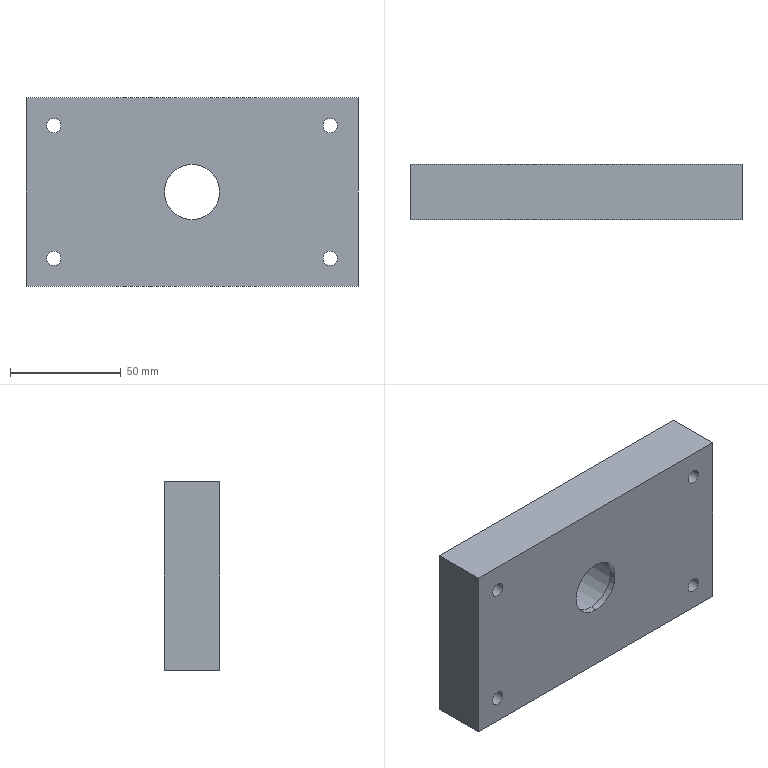Part | NX | features BREP 1 | 1 solid | 31 faces | box 150 x 25 x 85 mm | volume 290555 mm3 | cylinder 20 | plane 11 | commonest cylinder face diameters 6.5 x8 12 x8 25 x2 35 x2
STEP:
#1=CARTESIAN_POINT('',(-75.,0.,-42.5));
#2=VERTEX_POINT('',#1);
#3=CARTESIAN_POINT('',(-75.,0.,42.5));
#4=VERTEX_POINT('',#3);
#5=CARTESIAN_POINT('',(-75.,0.,-42.5));
#6=DIRECTION('',(0.,0.,1.));
#7=VECTOR('',#6,1000.);
#8=LINE('',#5,#7);
#9=EDGE_CURVE('',#2,#4,#8,.T.);
#10=ORIENTED_EDGE('',*,*,#9,.F.);
#11=CARTESIAN_POINT('',(75.,0.,-42.5));
#12=VERTEX_POINT('',#11);
#13=CARTESIAN_POINT('',(75.,0.,-42.5));
#14=DIRECTION('',(-1.,0.,0.));
#15=VECTOR('',#14,1000.);
#16=LINE('',#13,#15);
#17=EDGE_CURVE('',#12,#2,#16,.T.);
#18=ORIENTED_EDGE('',*,*,#17,.F.);
#19=CARTESIAN_POINT('',(75.,0.,42.5));
#20=VERTEX_POINT('',#19);
#21=CARTESIAN_POINT('',(75.,0.,42.5));
#22=DIRECTION('',(0.,0.,-1.));
#23=VECTOR('',#22,1000.);
#24=LINE('',#21,#23);
#25=EDGE_CURVE('',#20,#12,#24,.T.);
#26=ORIENTED_EDGE('',*,*,#25,.F.);
#27=CARTESIAN_POINT('',(-75.,0.,42.5));
#28=DIRECTION('',(1.,0.,0.));
#29=VECTOR('',#28,1000.);
#30=LINE('',#27,#29);
#31=EDGE_CURVE('',#4,#20,#30,.T.);
#32=ORIENTED_EDGE('',*,*,#31,.F.);
#33=EDGE_LOOP('',(#10,#18,#26,#32));
#34=FACE_BOUND('',#33,.T.);
#35=CARTESIAN_POINT('',(-65.75,0.,30.));
#36=VERTEX_POINT('',#35);
#37=CARTESIAN_POINT('',(-59.25,0.,30.));
#38=VERTEX_POINT('',#37);
#39=CARTESIAN_POINT('',(-62.5,0.,30.));
#40=DIRECTION('',(0.,1.,0.));
#41=DIRECTION('',(-1.,0.,0.));
#42=AXIS2_PLACEMENT_3D('',#39,#40,#41);
#43=CIRCLE('',#42,3.25);
#44=EDGE_CURVE('',#36,#38,#43,.T.);
#45=ORIENTED_EDGE('',*,*,#44,.T.);
#46=CARTESIAN_POINT('',(-62.5,0.,30.));
#47=DIRECTION('',(0.,1.,0.));
#48=DIRECTION('',(1.,0.,0.));
#49=AXIS2_PLACEMENT_3D('',#46,#47,#48);
#50=CIRCLE('',#49,3.25);
#51=EDGE_CURVE('',#38,#36,#50,.T.);
#52=ORIENTED_EDGE('',*,*,#51,.T.);
#53=EDGE_LOOP('',(#45,#52));
#54=FACE_BOUND('',#53,.T.);
#55=CARTESIAN_POINT('',(-65.75,0.,-30.));
#56=VERTEX_POINT('',#55);
#57=CARTESIAN_POINT('',(-59.25,0.,-30.));
#58=VERTEX_POINT('',#57);
#59=CARTESIAN_POINT('',(-62.5,0.,-30.));
#60=DIRECTION('',(0.,1.,0.));
#61=DIRECTION('',(-1.,0.,0.));
#62=AXIS2_PLACEMENT_3D('',#59,#60,#61);
#63=CIRCLE('',#62,3.25);
#64=EDGE_CURVE('',#56,#58,#63,.T.);
#65=ORIENTED_EDGE('',*,*,#64,.T.);
#66=CARTESIAN_POINT('',(-62.5,0.,-30.));
#67=DIRECTION('',(0.,1.,0.));
#68=DIRECTION('',(1.,0.,0.));
#69=AXIS2_PLACEMENT_3D('',#66,#67,#68);
#70=CIRCLE('',#69,3.25);
#71=EDGE_CURVE('',#58,#56,#70,.T.);
#72=ORIENTED_EDGE('',*,*,#71,.T.);
#73=EDGE_LOOP('',(#65,#72));
#74=FACE_BOUND('',#73,.T.);
#75=CARTESIAN_POINT('',(59.25,0.,30.));
#76=VERTEX_POINT('',#75);
#77=CARTESIAN_POINT('',(65.75,0.,30.));
#78=VERTEX_POINT('',#77);
#79=CARTESIAN_POINT('',(62.5,0.,30.));
#80=DIRECTION('',(0.,1.,0.));
#81=DIRECTION('',(-1.,0.,0.));
#82=AXIS2_PLACEMENT_3D('',#79,#80,#81);
#83=CIRCLE('',#82,3.25);
#84=EDGE_CURVE('',#76,#78,#83,.T.);
#85=ORIENTED_EDGE('',*,*,#84,.T.);
#86=CARTESIAN_POINT('',(62.5,0.,30.));
#87=DIRECTION('',(0.,1.,0.));
#88=DIRECTION('',(1.,0.,0.));
#89=AXIS2_PLACEMENT_3D('',#86,#87,#88);
#90=CIRCLE('',#89,3.25);
#91=EDGE_CURVE('',#78,#76,#90,.T.);
#92=ORIENTED_EDGE('',*,*,#91,.T.);
#93=EDGE_LOOP('',(#85,#92));
#94=FACE_BOUND('',#93,.T.);
#95=CARTESIAN_POINT('',(59.25,0.,-30.));
#96=VERTEX_POINT('',#95);
#97=CARTESIAN_POINT('',(65.75,0.,-30.));
#98=VERTEX_POINT('',#97);
#99=CARTESIAN_POINT('',(62.5,0.,-30.));
#100=DIRECTION('',(0.,1.,0.));
#101=DIRECTION('',(-1.,0.,0.));
#102=AXIS2_PLACEMENT_3D('',#99,#100,#101);
#103=CIRCLE('',#102,3.25);
#104=EDGE_CURVE('',#96,#98,#103,.T.);
#105=ORIENTED_EDGE('',*,*,#104,.T.);
#106=CARTESIAN_POINT('',(62.5,0.,-30.));
#107=DIRECTION('',(0.,1.,0.));
#108=DIRECTION('',(1.,0.,0.));
#109=AXIS2_PLACEMENT_3D('',#106,#107,#108);
#110=CIRCLE('',#109,3.25);
#111=EDGE_CURVE('',#98,#96,#110,.T.);
#112=ORIENTED_EDGE('',*,*,#111,.T.);
#113=EDGE_LOOP('',(#105,#112));
#114=FACE_BOUND('',#113,.T.);
#115=CARTESIAN_POINT('',(0.,0.,12.5));
#116=VERTEX_POINT('',#115);
#117=CARTESIAN_POINT('',(0.,0.,-12.5));
#118=VERTEX_POINT('',#117);
#119=CARTESIAN_POINT('',(0.,0.,0.));
#120=DIRECTION('',(0.,1.,0.));
#121=DIRECTION('',(0.,0.,1.));
#122=AXIS2_PLACEMENT_3D('',#119,#120,#121);
#123=CIRCLE('',#122,12.5);
#124=EDGE_CURVE('',#116,#118,#123,.T.);
#125=ORIENTED_EDGE('',*,*,#124,.T.);
#126=CARTESIAN_POINT('',(0.,0.,0.));
#127=DIRECTION('',(0.,1.,0.));
#128=DIRECTION('',(0.,0.,-1.));
#129=AXIS2_PLACEMENT_3D('',#126,#127,#128);
#130=CIRCLE('',#129,12.5);
#131=EDGE_CURVE('',#118,#116,#130,.T.);
#132=ORIENTED_EDGE('',*,*,#131,.T.);
#133=EDGE_LOOP('',(#125,#132));
#134=FACE_BOUND('',#133,.T.);
#135=CARTESIAN_POINT('',(0.,0.,0.));
#136=DIRECTION('',(0.,1.,0.));
#137=DIRECTION('',(1.,0.,0.));
#138=AXIS2_PLACEMENT_3D('',#135,#136,#137);
#139=PLANE('',#138);
#140=ADVANCED_FACE('',(#34,#54,#74,#94,#114,#134),#139,.F.);
#141=CARTESIAN_POINT('',(75.,25.,42.5));
#142=VERTEX_POINT('',#141);
#143=CARTESIAN_POINT('',(75.,0.,42.5));
#144=DIRECTION('',(0.,1.,0.));
#145=VECTOR('',#144,1000.);
#146=LINE('',#143,#145);
#147=EDGE_CURVE('',#20,#142,#146,.T.);
#148=ORIENTED_EDGE('',*,*,#147,.T.);
#149=CARTESIAN_POINT('',(-75.,25.,42.5));
#150=VERTEX_POINT('',#149);
#151=CARTESIAN_POINT('',(-75.,25.,42.5));
#152=DIRECTION('',(1.,0.,0.));
#153=VECTOR('',#152,1000.);
#154=LINE('',#151,#153);
#155=EDGE_CURVE('',#150,#142,#154,.T.);
#156=ORIENTED_EDGE('',*,*,#155,.F.);
#157=CARTESIAN_POINT('',(-75.,0.,42.5));
#158=DIRECTION('',(0.,1.,0.));
#159=VECTOR('',#158,1000.);
#160=LINE('',#157,#159);
#161=EDGE_CURVE('',#4,#150,#160,.T.);
#162=ORIENTED_EDGE('',*,*,#161,.F.);
#163=ORIENTED_EDGE('',*,*,#31,.T.);
#164=EDGE_LOOP('',(#148,#156,#162,#163));
#165=FACE_BOUND('',#164,.T.);
#166=CARTESIAN_POINT('',(-75.,0.,42.5));
#167=DIRECTION('',(0.,0.,1.));
#168=DIRECTION('',(1.,0.,0.));
#169=AXIS2_PLACEMENT_3D('',#166,#167,#168);
#170=PLANE('',#169);
#171=ADVANCED_FACE('',(#165),#170,.T.);
#172=ORIENTED_EDGE('',*,*,#161,.T.);
#173=CARTESIAN_POINT('',(-75.,25.,-42.5));
#174=VERTEX_POINT('',#173);
#175=CARTESIAN_POINT('',(-75.,25.,-42.5));
#176=DIRECTION('',(0.,0.,1.));
#177=VECTOR('',#176,1000.);
#178=LINE('',#175,#177);
#179=EDGE_CURVE('',#174,#150,#178,.T.);
#180=ORIENTED_EDGE('',*,*,#179,.F.);
#181=CARTESIAN_POINT('',(-75.,0.,-42.5));
#182=DIRECTION('',(0.,1.,0.));
#183=VECTOR('',#182,1000.);
#184=LINE('',#181,#183);
#185=EDGE_CURVE('',#2,#174,#184,.T.);
#186=ORIENTED_EDGE('',*,*,#185,.F.);
#187=ORIENTED_EDGE('',*,*,#9,.T.);
#188=EDGE_LOOP('',(#172,#180,#186,#187));
#189=FACE_BOUND('',#188,.T.);
#190=CARTESIAN_POINT('',(-75.,0.,-42.5));
#191=DIRECTION('',(-1.,0.,0.));
#192=DIRECTION('',(0.,0.,1.));
#193=AXIS2_PLACEMENT_3D('',#190,#191,#192);
#194=PLANE('',#193);
#195=ADVANCED_FACE('',(#189),#194,.T.);
#196=ORIENTED_EDGE('',*,*,#185,.T.);
#197=CARTESIAN_POINT('',(75.,25.,-42.5));
#198=VERTEX_POINT('',#197);
#199=CARTESIAN_POINT('',(75.,25.,-42.5));
#200=DIRECTION('',(-1.,0.,0.));
#201=VECTOR('',#200,1000.);
#202=LINE('',#199,#201);
#203=EDGE_CURVE('',#198,#174,#202,.T.);
#204=ORIENTED_EDGE('',*,*,#203,.F.);
#205=CARTESIAN_POINT('',(75.,0.,-42.5));
#206=DIRECTION('',(0.,1.,0.));
#207=VECTOR('',#206,1000.);
#208=LINE('',#205,#207);
#209=EDGE_CURVE('',#12,#198,#208,.T.);
#210=ORIENTED_EDGE('',*,*,#209,.F.);
#211=ORIENTED_EDGE('',*,*,#17,.T.);
#212=EDGE_LOOP('',(#196,#204,#210,#211));
#213=FACE_BOUND('',#212,.T.);
#214=CARTESIAN_POINT('',(75.,0.,-42.5));
#215=DIRECTION('',(0.,0.,-1.));
#216=DIRECTION('',(0.,-1.,0.));
#217=AXIS2_PLACEMENT_3D('',#214,#215,#216);
#218=PLANE('',#217);
#219=ADVANCED_FACE('',(#213),#218,.T.);
#220=ORIENTED_EDGE('',*,*,#209,.T.);
#221=CARTESIAN_POINT('',(75.,25.,42.5));
#222=DIRECTION('',(0.,0.,-1.));
#223=VECTOR('',#222,1000.);
#224=LINE('',#221,#223);
#225=EDGE_CURVE('',#142,#198,#224,.T.);
#226=ORIENTED_EDGE('',*,*,#225,.F.);
#227=ORIENTED_EDGE('',*,*,#147,.F.);
#228=ORIENTED_EDGE('',*,*,#25,.T.);
#229=EDGE_LOOP('',(#220,#226,#227,#228));
#230=FACE_BOUND('',#229,.T.);
#231=CARTESIAN_POINT('',(75.,0.,42.5));
#232=DIRECTION('',(1.,0.,0.));
#233=DIRECTION('',(0.,1.,0.));
#234=AXIS2_PLACEMENT_3D('',#231,#232,#233);
#235=PLANE('',#234);
#236=ADVANCED_FACE('',(#230),#235,.T.);
#237=ORIENTED_EDGE('',*,*,#225,.T.);
#238=ORIENTED_EDGE('',*,*,#203,.T.);
#239=ORIENTED_EDGE('',*,*,#179,.T.);
#240=ORIENTED_EDGE('',*,*,#155,.T.);
#241=EDGE_LOOP('',(#237,#238,#239,#240));
#242=FACE_BOUND('',#241,.T.);
#243=CARTESIAN_POINT('',(-68.5,25.,30.));
#244=VERTEX_POINT('',#243);
#245=CARTESIAN_POINT('',(-56.5,25.,30.));
#246=VERTEX_POINT('',#245);
#247=CARTESIAN_POINT('',(-62.5,25.,30.));
#248=DIRECTION('',(0.,1.,0.));
#249=DIRECTION('',(-1.,0.,0.));
#250=AXIS2_PLACEMENT_3D('',#247,#248,#249);
#251=CIRCLE('',#250,6.);
#252=EDGE_CURVE('',#244,#246,#251,.T.);
#253=ORIENTED_EDGE('',*,*,#252,.F.);
#254=CARTESIAN_POINT('',(-62.5,25.,30.));
#255=DIRECTION('',(0.,1.,0.));
#256=DIRECTION('',(1.,0.,0.));
#257=AXIS2_PLACEMENT_3D('',#254,#255,#256);
#258=CIRCLE('',#257,6.);
#259=EDGE_CURVE('',#246,#244,#258,.T.);
#260=ORIENTED_EDGE('',*,*,#259,.F.);
#261=EDGE_LOOP('',(#253,#260));
#262=FACE_BOUND('',#261,.T.);
#263=CARTESIAN_POINT('',(-68.5,25.,-30.));
#264=VERTEX_POINT('',#263);
#265=CARTESIAN_POINT('',(-56.5,25.,-30.));
#266=VERTEX_POINT('',#265);
#267=CARTESIAN_POINT('',(-62.5,25.,-30.));
#268=DIRECTION('',(0.,1.,0.));
#269=DIRECTION('',(-1.,0.,0.));
#270=AXIS2_PLACEMENT_3D('',#267,#268,#269);
#271=CIRCLE('',#270,6.);
#272=EDGE_CURVE('',#264,#266,#271,.T.);
#273=ORIENTED_EDGE('',*,*,#272,.F.);
#274=CARTESIAN_POINT('',(-62.5,25.,-30.));
#275=DIRECTION('',(0.,1.,0.));
#276=DIRECTION('',(1.,0.,0.));
#277=AXIS2_PLACEMENT_3D('',#274,#275,#276);
#278=CIRCLE('',#277,6.);
#279=EDGE_CURVE('',#266,#264,#278,.T.);
#280=ORIENTED_EDGE('',*,*,#279,.F.);
#281=EDGE_LOOP('',(#273,#280));
#282=FACE_BOUND('',#281,.T.);
#283=CARTESIAN_POINT('',(56.5,25.,30.));
#284=VERTEX_POINT('',#283);
#285=CARTESIAN_POINT('',(68.5,25.,30.));
#286=VERTEX_POINT('',#285);
#287=CARTESIAN_POINT('',(62.5,25.,30.));
#288=DIRECTION('',(0.,1.,0.));
#289=DIRECTION('',(-1.,0.,0.));
#290=AXIS2_PLACEMENT_3D('',#287,#288,#289);
#291=CIRCLE('',#290,6.);
#292=EDGE_CURVE('',#284,#286,#291,.T.);
#293=ORIENTED_EDGE('',*,*,#292,.F.);
#294=CARTESIAN_POINT('',(62.5,25.,30.));
#295=DIRECTION('',(0.,1.,0.));
#296=DIRECTION('',(1.,0.,0.));
#297=AXIS2_PLACEMENT_3D('',#294,#295,#296);
#298=CIRCLE('',#297,6.);
#299=EDGE_CURVE('',#286,#284,#298,.T.);
#300=ORIENTED_EDGE('',*,*,#299,.F.);
#301=EDGE_LOOP('',(#293,#300));
#302=FACE_BOUND('',#301,.T.);
#303=CARTESIAN_POINT('',(56.5,25.,-30.));
#304=VERTEX_POINT('',#303);
#305=CARTESIAN_POINT('',(68.5,25.,-30.));
#306=VERTEX_POINT('',#305);
#307=CARTESIAN_POINT('',(62.5,25.,-30.));
#308=DIRECTION('',(0.,1.,0.));
#309=DIRECTION('',(-1.,0.,0.));
#310=AXIS2_PLACEMENT_3D('',#307,#308,#309);
#311=CIRCLE('',#310,6.);
#312=EDGE_CURVE('',#304,#306,#311,.T.);
#313=ORIENTED_EDGE('',*,*,#312,.F.);
#314=CARTESIAN_POINT('',(62.5,25.,-30.));
#315=DIRECTION('',(0.,1.,0.));
#316=DIRECTION('',(1.,0.,0.));
#317=AXIS2_PLACEMENT_3D('',#314,#315,#316);
#318=CIRCLE('',#317,6.);
#319=EDGE_CURVE('',#306,#304,#318,.T.);
#320=ORIENTED_EDGE('',*,*,#319,.F.);
#321=EDGE_LOOP('',(#313,#320));
#322=FACE_BOUND('',#321,.T.);
#323=CARTESIAN_POINT('',(0.,25.,17.5));
#324=VERTEX_POINT('',#323);
#325=CARTESIAN_POINT('',(0.,25.,-17.5));
#326=VERTEX_POINT('',#325);
#327=CARTESIAN_POINT('',(0.,25.,0.));
#328=DIRECTION('',(0.,1.,0.));
#329=DIRECTION('',(0.,0.,1.));
#330=AXIS2_PLACEMENT_3D('',#327,#328,#329);
#331=CIRCLE('',#330,17.5);
#332=EDGE_CURVE('',#324,#326,#331,.T.);
#333=ORIENTED_EDGE('',*,*,#332,.F.);
#334=CARTESIAN_POINT('',(0.,25.,0.));
#335=DIRECTION('',(0.,1.,0.));
#336=DIRECTION('',(0.,0.,-1.));
#337=AXIS2_PLACEMENT_3D('',#334,#335,#336);
#338=CIRCLE('',#337,17.5);
#339=EDGE_CURVE('',#326,#324,#338,.T.);
#340=ORIENTED_EDGE('',*,*,#339,.F.);
#341=EDGE_LOOP('',(#333,#340));
#342=FACE_BOUND('',#341,.T.);
#343=CARTESIAN_POINT('',(0.,25.,0.));
#344=DIRECTION('',(0.,1.,0.));
#345=DIRECTION('',(1.,0.,0.));
#346=AXIS2_PLACEMENT_3D('',#343,#344,#345);
#347=PLANE('',#346);
#348=ADVANCED_FACE('',(#242,#262,#282,#302,#322,#342),#347,.T.);
#349=CARTESIAN_POINT('',(-68.5,18.,30.));
#350=VERTEX_POINT('',#349);
#351=CARTESIAN_POINT('',(-68.5,18.,30.));
#352=DIRECTION('',(0.,1.,0.));
#353=VECTOR('',#352,1000.);
#354=LINE('',#351,#353);
#355=EDGE_CURVE('',#350,#244,#354,.T.);
#356=ORIENTED_EDGE('',*,*,#355,.F.);
#357=CARTESIAN_POINT('',(-56.5,18.,30.));
#358=VERTEX_POINT('',#357);
#359=CARTESIAN_POINT('',(-62.5,18.,30.));
#360=DIRECTION('',(0.,1.,0.));
#361=DIRECTION('',(1.,0.,0.));
#362=AXIS2_PLACEMENT_3D('',#359,#360,#361);
#363=CIRCLE('',#362,6.);
#364=EDGE_CURVE('',#358,#350,#363,.T.);
#365=ORIENTED_EDGE('',*,*,#364,.F.);
#366=CARTESIAN_POINT('',(-56.5,18.,30.));
#367=DIRECTION('',(0.,1.,0.));
#368=VECTOR('',#367,1000.);
#369=LINE('',#366,#368);
#370=EDGE_CURVE('',#358,#246,#369,.T.);
#371=ORIENTED_EDGE('',*,*,#370,.T.);
#372=ORIENTED_EDGE('',*,*,#259,.T.);
#373=EDGE_LOOP('',(#356,#365,#371,#372));
#374=FACE_BOUND('',#373,.T.);
#375=CARTESIAN_POINT('',(-62.5,-19.544,30.));
#376=DIRECTION('',(0.,1.,0.));
#377=DIRECTION('',(1.,0.,0.));
#378=AXIS2_PLACEMENT_3D('',#375,#376,#377);
#379=CYLINDRICAL_SURFACE('',#378,6.);
#380=ADVANCED_FACE('',(#374),#379,.F.);
#381=ORIENTED_EDGE('',*,*,#370,.F.);
#382=CARTESIAN_POINT('',(-62.5,18.,30.));
#383=DIRECTION('',(0.,-1.,0.));
#384=DIRECTION('',(1.,0.,0.));
#385=AXIS2_PLACEMENT_3D('',#382,#383,#384);
#386=CIRCLE('',#385,6.);
#387=EDGE_CURVE('',#358,#350,#386,.T.);
#388=ORIENTED_EDGE('',*,*,#387,.T.);
#389=ORIENTED_EDGE('',*,*,#355,.T.);
#390=ORIENTED_EDGE('',*,*,#252,.T.);
#391=EDGE_LOOP('',(#381,#388,#389,#390));
#392=FACE_BOUND('',#391,.T.);
#393=CARTESIAN_POINT('',(-62.5,-19.544,30.));
#394=DIRECTION('',(0.,1.,0.));
#395=DIRECTION('',(1.,0.,0.));
#396=AXIS2_PLACEMENT_3D('',#393,#394,#395);
#397=CYLINDRICAL_SURFACE('',#396,6.);
#398=ADVANCED_FACE('',(#392),#397,.F.);
#399=ORIENTED_EDGE('',*,*,#387,.F.);
#400=ORIENTED_EDGE('',*,*,#364,.T.);
#401=EDGE_LOOP('',(#399,#400));
#402=FACE_BOUND('',#401,.T.);
#403=CARTESIAN_POINT('',(-59.25,18.,30.));
#404=VERTEX_POINT('',#403);
#405=CARTESIAN_POINT('',(-65.75,18.,30.));
#406=VERTEX_POINT('',#405);
#407=CARTESIAN_POINT('',(-62.5,18.,30.));
#408=DIRECTION('',(0.,1.,0.));
#409=DIRECTION('',(1.,0.,0.));
#410=AXIS2_PLACEMENT_3D('',#407,#408,#409);
#411=CIRCLE('',#410,3.25);
#412=EDGE_CURVE('',#404,#406,#411,.T.);
#413=ORIENTED_EDGE('',*,*,#412,.F.);
#414=CARTESIAN_POINT('',(-62.5,18.,30.));
#415=DIRECTION('',(0.,-1.,0.));
#416=DIRECTION('',(1.,0.,0.));
#417=AXIS2_PLACEMENT_3D('',#414,#415,#416);
#418=CIRCLE('',#417,3.25);
#419=EDGE_CURVE('',#404,#406,#418,.T.);
#420=ORIENTED_EDGE('',*,*,#419,.T.);
#421=EDGE_LOOP('',(#413,#420));
#422=FACE_BOUND('',#421,.T.);
#423=CARTESIAN_POINT('',(-62.5,18.,30.));
#424=DIRECTION('',(0.,1.,0.));
#425=DIRECTION('',(1.,0.,0.));
#426=AXIS2_PLACEMENT_3D('',#423,#424,#425);
#427=PLANE('',#426);
#428=ADVANCED_FACE('',(#402,#422),#427,.T.);
#429=CARTESIAN_POINT('',(-65.75,0.,30.));
#430=DIRECTION('',(0.,1.,0.));
#431=VECTOR('',#430,1000.);
#432=LINE('',#429,#431);
#433=EDGE_CURVE('',#36,#406,#432,.T.);
#434=ORIENTED_EDGE('',*,*,#433,.T.);
#435=ORIENTED_EDGE('',*,*,#419,.F.);
#436=CARTESIAN_POINT('',(-59.25,0.,30.));
#437=DIRECTION('',(0.,1.,0.));
#438=VECTOR('',#437,1000.);
#439=LINE('',#436,#438);
#440=EDGE_CURVE('',#38,#404,#439,.T.);
#441=ORIENTED_EDGE('',*,*,#440,.F.);
#442=ORIENTED_EDGE('',*,*,#44,.F.);
#443=EDGE_LOOP('',(#434,#435,#441,#442));
#444=FACE_BOUND('',#443,.T.);
#445=CARTESIAN_POINT('',(-62.5,-19.544,30.));
#446=DIRECTION('',(0.,1.,0.));
#447=DIRECTION('',(1.,0.,0.));
#448=AXIS2_PLACEMENT_3D('',#445,#446,#447);
#449=CYLINDRICAL_SURFACE('',#448,3.25);
#450=ADVANCED_FACE('',(#444),#449,.F.);
#451=ORIENTED_EDGE('',*,*,#440,.T.);
#452=ORIENTED_EDGE('',*,*,#412,.T.);
#453=ORIENTED_EDGE('',*,*,#433,.F.);
#454=ORIENTED_EDGE('',*,*,#51,.F.);
#455=EDGE_LOOP('',(#451,#452,#453,#454));
#456=FACE_BOUND('',#455,.T.);
#457=CARTESIAN_POINT('',(-62.5,-19.544,30.));
#458=DIRECTION('',(0.,1.,0.));
#459=DIRECTION('',(1.,0.,0.));
#460=AXIS2_PLACEMENT_3D('',#457,#458,#459);
#461=CYLINDRICAL_SURFACE('',#460,3.25);
#462=ADVANCED_FACE('',(#456),#461,.F.);
#463=CARTESIAN_POINT('',(-68.5,18.,-30.));
#464=VERTEX_POINT('',#463);
#465=CARTESIAN_POINT('',(-68.5,18.,-30.));
#466=DIRECTION('',(0.,1.,0.));
#467=VECTOR('',#466,1000.);
#468=LINE('',#465,#467);
#469=EDGE_CURVE('',#464,#264,#468,.T.);
#470=ORIENTED_EDGE('',*,*,#469,.F.);
#471=CARTESIAN_POINT('',(-56.5,18.,-30.));
#472=VERTEX_POINT('',#471);
#473=CARTESIAN_POINT('',(-62.5,18.,-30.));
#474=DIRECTION('',(0.,1.,0.));
#475=DIRECTION('',(1.,0.,0.));
#476=AXIS2_PLACEMENT_3D('',#473,#474,#475);
#477=CIRCLE('',#476,6.);
#478=EDGE_CURVE('',#472,#464,#477,.T.);
#479=ORIENTED_EDGE('',*,*,#478,.F.);
#480=CARTESIAN_POINT('',(-56.5,18.,-30.));
#481=DIRECTION('',(0.,1.,0.));
#482=VECTOR('',#481,1000.);
#483=LINE('',#480,#482);
#484=EDGE_CURVE('',#472,#266,#483,.T.);
#485=ORIENTED_EDGE('',*,*,#484,.T.);
#486=ORIENTED_EDGE('',*,*,#279,.T.);
#487=EDGE_LOOP('',(#470,#479,#485,#486));
#488=FACE_BOUND('',#487,.T.);
#489=CARTESIAN_POINT('',(-62.5,-19.544,-30.));
#490=DIRECTION('',(0.,1.,0.));
#491=DIRECTION('',(1.,0.,0.));
#492=AXIS2_PLACEMENT_3D('',#489,#490,#491);
#493=CYLINDRICAL_SURFACE('',#492,6.);
#494=ADVANCED_FACE('',(#488),#493,.F.);
#495=ORIENTED_EDGE('',*,*,#484,.F.);
#496=CARTESIAN_POINT('',(-62.5,18.,-30.));
#497=DIRECTION('',(0.,-1.,0.));
#498=DIRECTION('',(1.,0.,0.));
#499=AXIS2_PLACEMENT_3D('',#496,#497,#498);
#500=CIRCLE('',#499,6.);
#501=EDGE_CURVE('',#472,#464,#500,.T.);
#502=ORIENTED_EDGE('',*,*,#501,.T.);
#503=ORIENTED_EDGE('',*,*,#469,.T.);
#504=ORIENTED_EDGE('',*,*,#272,.T.);
#505=EDGE_LOOP('',(#495,#502,#503,#504));
#506=FACE_BOUND('',#505,.T.);
#507=CARTESIAN_POINT('',(-62.5,-19.544,-30.));
#508=DIRECTION('',(0.,1.,0.));
#509=DIRECTION('',(1.,0.,0.));
#510=AXIS2_PLACEMENT_3D('',#507,#508,#509);
#511=CYLINDRICAL_SURFACE('',#510,6.);
#512=ADVANCED_FACE('',(#506),#511,.F.);
#513=ORIENTED_EDGE('',*,*,#501,.F.);
#514=ORIENTED_EDGE('',*,*,#478,.T.);
#515=EDGE_LOOP('',(#513,#514));
#516=FACE_BOUND('',#515,.T.);
#517=CARTESIAN_POINT('',(-59.25,18.,-30.));
#518=VERTEX_POINT('',#517);
#519=CARTESIAN_POINT('',(-65.75,18.,-30.));
#520=VERTEX_POINT('',#519);
#521=CARTESIAN_POINT('',(-62.5,18.,-30.));
#522=DIRECTION('',(0.,1.,0.));
#523=DIRECTION('',(1.,0.,0.));
#524=AXIS2_PLACEMENT_3D('',#521,#522,#523);
#525=CIRCLE('',#524,3.25);
#526=EDGE_CURVE('',#518,#520,#525,.T.);
#527=ORIENTED_EDGE('',*,*,#526,.F.);
#528=CARTESIAN_POINT('',(-62.5,18.,-30.));
#529=DIRECTION('',(0.,-1.,0.));
#530=DIRECTION('',(1.,0.,0.));
#531=AXIS2_PLACEMENT_3D('',#528,#529,#530);
#532=CIRCLE('',#531,3.25);
#533=EDGE_CURVE('',#518,#520,#532,.T.);
#534=ORIENTED_EDGE('',*,*,#533,.T.);
#535=EDGE_LOOP('',(#527,#534));
#536=FACE_BOUND('',#535,.T.);
#537=CARTESIAN_POINT('',(-62.5,18.,-30.));
#538=DIRECTION('',(0.,1.,0.));
#539=DIRECTION('',(1.,0.,0.));
#540=AXIS2_PLACEMENT_3D('',#537,#538,#539);
#541=PLANE('',#540);
#542=ADVANCED_FACE('',(#516,#536),#541,.T.);
#543=CARTESIAN_POINT('',(-65.75,0.,-30.));
#544=DIRECTION('',(0.,1.,0.));
#545=VECTOR('',#544,1000.);
#546=LINE('',#543,#545);
#547=EDGE_CURVE('',#56,#520,#546,.T.);
#548=ORIENTED_EDGE('',*,*,#547,.T.);
#549=ORIENTED_EDGE('',*,*,#533,.F.);
#550=CARTESIAN_POINT('',(-59.25,0.,-30.));
#551=DIRECTION('',(0.,1.,0.));
#552=VECTOR('',#551,1000.);
#553=LINE('',#550,#552);
#554=EDGE_CURVE('',#58,#518,#553,.T.);
#555=ORIENTED_EDGE('',*,*,#554,.F.);
#556=ORIENTED_EDGE('',*,*,#64,.F.);
#557=EDGE_LOOP('',(#548,#549,#555,#556));
#558=FACE_BOUND('',#557,.T.);
#559=CARTESIAN_POINT('',(-62.5,-19.544,-30.));
#560=DIRECTION('',(0.,1.,0.));
#561=DIRECTION('',(1.,0.,0.));
#562=AXIS2_PLACEMENT_3D('',#559,#560,#561);
#563=CYLINDRICAL_SURFACE('',#562,3.25);
#564=ADVANCED_FACE('',(#558),#563,.F.);
#565=ORIENTED_EDGE('',*,*,#554,.T.);
#566=ORIENTED_EDGE('',*,*,#526,.T.);
#567=ORIENTED_EDGE('',*,*,#547,.F.);
#568=ORIENTED_EDGE('',*,*,#71,.F.);
#569=EDGE_LOOP('',(#565,#566,#567,#568));
#570=FACE_BOUND('',#569,.T.);
#571=CARTESIAN_POINT('',(-62.5,-19.544,-30.));
#572=DIRECTION('',(0.,1.,0.));
#573=DIRECTION('',(1.,0.,0.));
#574=AXIS2_PLACEMENT_3D('',#571,#572,#573);
#575=CYLINDRICAL_SURFACE('',#574,3.25);
#576=ADVANCED_FACE('',(#570),#575,.F.);
#577=CARTESIAN_POINT('',(56.5,18.,30.));
#578=VERTEX_POINT('',#577);
#579=CARTESIAN_POINT('',(56.5,18.,30.));
#580=DIRECTION('',(0.,1.,0.));
#581=VECTOR('',#580,1000.);
#582=LINE('',#579,#581);
#583=EDGE_CURVE('',#578,#284,#582,.T.);
#584=ORIENTED_EDGE('',*,*,#583,.F.);
#585=CARTESIAN_POINT('',(68.5,18.,30.));
#586=VERTEX_POINT('',#585);
#587=CARTESIAN_POINT('',(62.5,18.,30.));
#588=DIRECTION('',(0.,1.,0.));
#589=DIRECTION('',(1.,0.,0.));
#590=AXIS2_PLACEMENT_3D('',#587,#588,#589);
#591=CIRCLE('',#590,6.);
#592=EDGE_CURVE('',#586,#578,#591,.T.);
#593=ORIENTED_EDGE('',*,*,#592,.F.);
#594=CARTESIAN_POINT('',(68.5,18.,30.));
#595=DIRECTION('',(0.,1.,0.));
#596=VECTOR('',#595,1000.);
#597=LINE('',#594,#596);
#598=EDGE_CURVE('',#586,#286,#597,.T.);
#599=ORIENTED_EDGE('',*,*,#598,.T.);
#600=ORIENTED_EDGE('',*,*,#299,.T.);
#601=EDGE_LOOP('',(#584,#593,#599,#600));
#602=FACE_BOUND('',#601,.T.);
#603=CARTESIAN_POINT('',(62.5,-19.544,30.));
#604=DIRECTION('',(0.,1.,0.));
#605=DIRECTION('',(1.,0.,0.));
#606=AXIS2_PLACEMENT_3D('',#603,#604,#605);
#607=CYLINDRICAL_SURFACE('',#606,6.);
#608=ADVANCED_FACE('',(#602),#607,.F.);
#609=ORIENTED_EDGE('',*,*,#598,.F.);
#610=CARTESIAN_POINT('',(62.5,18.,30.));
#611=DIRECTION('',(0.,-1.,0.));
#612=DIRECTION('',(1.,0.,0.));
#613=AXIS2_PLACEMENT_3D('',#610,#611,#612);
#614=CIRCLE('',#613,6.);
#615=EDGE_CURVE('',#586,#578,#614,.T.);
#616=ORIENTED_EDGE('',*,*,#615,.T.);
#617=ORIENTED_EDGE('',*,*,#583,.T.);
#618=ORIENTED_EDGE('',*,*,#292,.T.);
#619=EDGE_LOOP('',(#609,#616,#617,#618));
#620=FACE_BOUND('',#619,.T.);
#621=CARTESIAN_POINT('',(62.5,-19.544,30.));
#622=DIRECTION('',(0.,1.,0.));
#623=DIRECTION('',(1.,0.,0.));
#624=AXIS2_PLACEMENT_3D('',#621,#622,#623);
#625=CYLINDRICAL_SURFACE('',#624,6.);
#626=ADVANCED_FACE('',(#620),#625,.F.);
#627=ORIENTED_EDGE('',*,*,#615,.F.);
#628=ORIENTED_EDGE('',*,*,#592,.T.);
#629=EDGE_LOOP('',(#627,#628));
#630=FACE_BOUND('',#629,.T.);
#631=CARTESIAN_POINT('',(65.75,18.,30.));
#632=VERTEX_POINT('',#631);
#633=CARTESIAN_POINT('',(59.25,18.,30.));
#634=VERTEX_POINT('',#633);
#635=CARTESIAN_POINT('',(62.5,18.,30.));
#636=DIRECTION('',(0.,1.,0.));
#637=DIRECTION('',(1.,0.,0.));
#638=AXIS2_PLACEMENT_3D('',#635,#636,#637);
#639=CIRCLE('',#638,3.25);
#640=EDGE_CURVE('',#632,#634,#639,.T.);
#641=ORIENTED_EDGE('',*,*,#640,.F.);
#642=CARTESIAN_POINT('',(62.5,18.,30.));
#643=DIRECTION('',(0.,-1.,0.));
#644=DIRECTION('',(1.,0.,0.));
#645=AXIS2_PLACEMENT_3D('',#642,#643,#644);
#646=CIRCLE('',#645,3.25);
#647=EDGE_CURVE('',#632,#634,#646,.T.);
#648=ORIENTED_EDGE('',*,*,#647,.T.);
#649=EDGE_LOOP('',(#641,#648));
#650=FACE_BOUND('',#649,.T.);
#651=CARTESIAN_POINT('',(62.5,18.,30.));
#652=DIRECTION('',(0.,1.,0.));
#653=DIRECTION('',(1.,0.,0.));
#654=AXIS2_PLACEMENT_3D('',#651,#652,#653);
#655=PLANE('',#654);
#656=ADVANCED_FACE('',(#630,#650),#655,.T.);
#657=CARTESIAN_POINT('',(59.25,0.,30.));
#658=DIRECTION('',(0.,1.,0.));
#659=VECTOR('',#658,1000.);
#660=LINE('',#657,#659);
#661=EDGE_CURVE('',#76,#634,#660,.T.);
#662=ORIENTED_EDGE('',*,*,#661,.T.);
#663=ORIENTED_EDGE('',*,*,#647,.F.);
#664=CARTESIAN_POINT('',(65.75,0.,30.));
#665=DIRECTION('',(0.,1.,0.));
#666=VECTOR('',#665,1000.);
#667=LINE('',#664,#666);
#668=EDGE_CURVE('',#78,#632,#667,.T.);
#669=ORIENTED_EDGE('',*,*,#668,.F.);
#670=ORIENTED_EDGE('',*,*,#84,.F.);
#671=EDGE_LOOP('',(#662,#663,#669,#670));
#672=FACE_BOUND('',#671,.T.);
#673=CARTESIAN_POINT('',(62.5,-19.544,30.));
#674=DIRECTION('',(0.,1.,0.));
#675=DIRECTION('',(1.,0.,0.));
#676=AXIS2_PLACEMENT_3D('',#673,#674,#675);
#677=CYLINDRICAL_SURFACE('',#676,3.25);
#678=ADVANCED_FACE('',(#672),#677,.F.);
#679=ORIENTED_EDGE('',*,*,#668,.T.);
#680=ORIENTED_EDGE('',*,*,#640,.T.);
#681=ORIENTED_EDGE('',*,*,#661,.F.);
#682=ORIENTED_EDGE('',*,*,#91,.F.);
#683=EDGE_LOOP('',(#679,#680,#681,#682));
#684=FACE_BOUND('',#683,.T.);
#685=CARTESIAN_POINT('',(62.5,-19.544,30.));
#686=DIRECTION('',(0.,1.,0.));
#687=DIRECTION('',(1.,0.,0.));
#688=AXIS2_PLACEMENT_3D('',#685,#686,#687);
#689=CYLINDRICAL_SURFACE('',#688,3.25);
#690=ADVANCED_FACE('',(#684),#689,.F.);
#691=CARTESIAN_POINT('',(56.5,18.,-30.));
#692=VERTEX_POINT('',#691);
#693=CARTESIAN_POINT('',(56.5,18.,-30.));
#694=DIRECTION('',(0.,1.,0.));
#695=VECTOR('',#694,1000.);
#696=LINE('',#693,#695);
#697=EDGE_CURVE('',#692,#304,#696,.T.);
#698=ORIENTED_EDGE('',*,*,#697,.F.);
#699=CARTESIAN_POINT('',(68.5,18.,-30.));
#700=VERTEX_POINT('',#699);
#701=CARTESIAN_POINT('',(62.5,18.,-30.));
#702=DIRECTION('',(0.,1.,0.));
#703=DIRECTION('',(1.,0.,0.));
#704=AXIS2_PLACEMENT_3D('',#701,#702,#703);
#705=CIRCLE('',#704,6.);
#706=EDGE_CURVE('',#700,#692,#705,.T.);
#707=ORIENTED_EDGE('',*,*,#706,.F.);
#708=CARTESIAN_POINT('',(68.5,18.,-30.));
#709=DIRECTION('',(0.,1.,0.));
#710=VECTOR('',#709,1000.);
#711=LINE('',#708,#710);
#712=EDGE_CURVE('',#700,#306,#711,.T.);
#713=ORIENTED_EDGE('',*,*,#712,.T.);
#714=ORIENTED_EDGE('',*,*,#319,.T.);
#715=EDGE_LOOP('',(#698,#707,#713,#714));
#716=FACE_BOUND('',#715,.T.);
#717=CARTESIAN_POINT('',(62.5,-19.544,-30.));
#718=DIRECTION('',(0.,1.,0.));
#719=DIRECTION('',(1.,0.,0.));
#720=AXIS2_PLACEMENT_3D('',#717,#718,#719);
#721=CYLINDRICAL_SURFACE('',#720,6.);
#722=ADVANCED_FACE('',(#716),#721,.F.);
#723=ORIENTED_EDGE('',*,*,#712,.F.);
#724=CARTESIAN_POINT('',(62.5,18.,-30.));
#725=DIRECTION('',(0.,-1.,0.));
#726=DIRECTION('',(1.,0.,0.));
#727=AXIS2_PLACEMENT_3D('',#724,#725,#726);
#728=CIRCLE('',#727,6.);
#729=EDGE_CURVE('',#700,#692,#728,.T.);
#730=ORIENTED_EDGE('',*,*,#729,.T.);
#731=ORIENTED_EDGE('',*,*,#697,.T.);
#732=ORIENTED_EDGE('',*,*,#312,.T.);
#733=EDGE_LOOP('',(#723,#730,#731,#732));
#734=FACE_BOUND('',#733,.T.);
#735=CARTESIAN_POINT('',(62.5,-19.544,-30.));
#736=DIRECTION('',(0.,1.,0.));
#737=DIRECTION('',(1.,0.,0.));
#738=AXIS2_PLACEMENT_3D('',#735,#736,#737);
#739=CYLINDRICAL_SURFACE('',#738,6.);
#740=ADVANCED_FACE('',(#734),#739,.F.);
#741=ORIENTED_EDGE('',*,*,#729,.F.);
#742=ORIENTED_EDGE('',*,*,#706,.T.);
#743=EDGE_LOOP('',(#741,#742));
#744=FACE_BOUND('',#743,.T.);
#745=CARTESIAN_POINT('',(65.75,18.,-30.));
#746=VERTEX_POINT('',#745);
#747=CARTESIAN_POINT('',(59.25,18.,-30.));
#748=VERTEX_POINT('',#747);
#749=CARTESIAN_POINT('',(62.5,18.,-30.));
#750=DIRECTION('',(0.,1.,0.));
#751=DIRECTION('',(1.,0.,0.));
#752=AXIS2_PLACEMENT_3D('',#749,#750,#751);
#753=CIRCLE('',#752,3.25);
#754=EDGE_CURVE('',#746,#748,#753,.T.);
#755=ORIENTED_EDGE('',*,*,#754,.F.);
#756=CARTESIAN_POINT('',(62.5,18.,-30.));
#757=DIRECTION('',(0.,-1.,0.));
#758=DIRECTION('',(1.,0.,0.));
#759=AXIS2_PLACEMENT_3D('',#756,#757,#758);
#760=CIRCLE('',#759,3.25);
#761=EDGE_CURVE('',#746,#748,#760,.T.);
#762=ORIENTED_EDGE('',*,*,#761,.T.);
#763=EDGE_LOOP('',(#755,#762));
#764=FACE_BOUND('',#763,.T.);
#765=CARTESIAN_POINT('',(62.5,18.,-30.));
#766=DIRECTION('',(0.,1.,0.));
#767=DIRECTION('',(1.,0.,0.));
#768=AXIS2_PLACEMENT_3D('',#765,#766,#767);
#769=PLANE('',#768);
#770=ADVANCED_FACE('',(#744,#764),#769,.T.);
#771=CARTESIAN_POINT('',(59.25,0.,-30.));
#772=DIRECTION('',(0.,1.,0.));
#773=VECTOR('',#772,1000.);
#774=LINE('',#771,#773);
#775=EDGE_CURVE('',#96,#748,#774,.T.);
#776=ORIENTED_EDGE('',*,*,#775,.T.);
#777=ORIENTED_EDGE('',*,*,#761,.F.);
#778=CARTESIAN_POINT('',(65.75,0.,-30.));
#779=DIRECTION('',(0.,1.,0.));
#780=VECTOR('',#779,1000.);
#781=LINE('',#778,#780);
#782=EDGE_CURVE('',#98,#746,#781,.T.);
#783=ORIENTED_EDGE('',*,*,#782,.F.);
#784=ORIENTED_EDGE('',*,*,#104,.F.);
#785=EDGE_LOOP('',(#776,#777,#783,#784));
#786=FACE_BOUND('',#785,.T.);
#787=CARTESIAN_POINT('',(62.5,-19.544,-30.));
#788=DIRECTION('',(0.,1.,0.));
#789=DIRECTION('',(1.,0.,0.));
#790=AXIS2_PLACEMENT_3D('',#787,#788,#789);
#791=CYLINDRICAL_SURFACE('',#790,3.25);
#792=ADVANCED_FACE('',(#786),#791,.F.);
#793=ORIENTED_EDGE('',*,*,#782,.T.);
#794=ORIENTED_EDGE('',*,*,#754,.T.);
#795=ORIENTED_EDGE('',*,*,#775,.F.);
#796=ORIENTED_EDGE('',*,*,#111,.F.);
#797=EDGE_LOOP('',(#793,#794,#795,#796));
#798=FACE_BOUND('',#797,.T.);
#799=CARTESIAN_POINT('',(62.5,-19.544,-30.));
#800=DIRECTION('',(0.,1.,0.));
#801=DIRECTION('',(1.,0.,0.));
#802=AXIS2_PLACEMENT_3D('',#799,#800,#801);
#803=CYLINDRICAL_SURFACE('',#802,3.25);
#804=ADVANCED_FACE('',(#798),#803,.F.);
#805=CARTESIAN_POINT('',(0.,3.,17.5));
#806=VERTEX_POINT('',#805);
#807=CARTESIAN_POINT('',(0.,25.,17.5));
#808=DIRECTION('',(0.,-1.,0.));
#809=VECTOR('',#808,1000.);
#810=LINE('',#807,#809);
#811=EDGE_CURVE('',#806,#324,#810,.F.);
#812=ORIENTED_EDGE('',*,*,#811,.F.);
#813=CARTESIAN_POINT('',(0.,3.,-17.5));
#814=VERTEX_POINT('',#813);
#815=CARTESIAN_POINT('',(0.,3.,0.));
#816=DIRECTION('',(0.,1.,0.));
#817=DIRECTION('',(0.,0.,-1.));
#818=AXIS2_PLACEMENT_3D('',#815,#816,#817);
#819=CIRCLE('',#818,17.5);
#820=EDGE_CURVE('',#814,#806,#819,.T.);
#821=ORIENTED_EDGE('',*,*,#820,.F.);
#822=CARTESIAN_POINT('',(0.,25.,-17.5));
#823=DIRECTION('',(0.,-1.,0.));
#824=VECTOR('',#823,1000.);
#825=LINE('',#822,#824);
#826=EDGE_CURVE('',#814,#326,#825,.F.);
#827=ORIENTED_EDGE('',*,*,#826,.T.);
#828=ORIENTED_EDGE('',*,*,#339,.T.);
#829=EDGE_LOOP('',(#812,#821,#827,#828));
#830=FACE_BOUND('',#829,.T.);
#831=CARTESIAN_POINT('',(0.,25.,0.));
#832=DIRECTION('',(0.,1.,0.));
#833=DIRECTION('',(0.,0.,-1.));
#834=AXIS2_PLACEMENT_3D('',#831,#832,#833);
#835=CYLINDRICAL_SURFACE('',#834,17.5);
#836=ADVANCED_FACE('',(#830),#835,.F.);
#837=ORIENTED_EDGE('',*,*,#826,.F.);
#838=CARTESIAN_POINT('',(0.,3.,0.));
#839=DIRECTION('',(0.,1.,0.));
#840=DIRECTION('',(0.,0.,1.));
#841=AXIS2_PLACEMENT_3D('',#838,#839,#840);
#842=CIRCLE('',#841,17.5);
#843=EDGE_CURVE('',#806,#814,#842,.T.);
#844=ORIENTED_EDGE('',*,*,#843,.F.);
#845=ORIENTED_EDGE('',*,*,#811,.T.);
#846=ORIENTED_EDGE('',*,*,#332,.T.);
#847=EDGE_LOOP('',(#837,#844,#845,#846));
#848=FACE_BOUND('',#847,.T.);
#849=CARTESIAN_POINT('',(0.,25.,0.));
#850=DIRECTION('',(0.,1.,0.));
#851=DIRECTION('',(0.,0.,-1.));
#852=AXIS2_PLACEMENT_3D('',#849,#850,#851);
#853=CYLINDRICAL_SURFACE('',#852,17.5);
#854=ADVANCED_FACE('',(#848),#853,.F.);
#855=ORIENTED_EDGE('',*,*,#843,.T.);
#856=ORIENTED_EDGE('',*,*,#820,.T.);
#857=EDGE_LOOP('',(#855,#856));
#858=FACE_BOUND('',#857,.T.);
#859=CARTESIAN_POINT('',(0.,3.,12.5));
#860=VERTEX_POINT('',#859);
#861=CARTESIAN_POINT('',(0.,3.,-12.5));
#862=VERTEX_POINT('',#861);
#863=CARTESIAN_POINT('',(0.,3.,0.));
#864=DIRECTION('',(0.,1.,0.));
#865=DIRECTION('',(0.,0.,1.));
#866=AXIS2_PLACEMENT_3D('',#863,#864,#865);
#867=CIRCLE('',#866,12.5);
#868=EDGE_CURVE('',#860,#862,#867,.T.);
#869=ORIENTED_EDGE('',*,*,#868,.F.);
#870=CARTESIAN_POINT('',(0.,3.,0.));
#871=DIRECTION('',(0.,1.,0.));
#872=DIRECTION('',(0.,0.,-1.));
#873=AXIS2_PLACEMENT_3D('',#870,#871,#872);
#874=CIRCLE('',#873,12.5);
#875=EDGE_CURVE('',#862,#860,#874,.T.);
#876=ORIENTED_EDGE('',*,*,#875,.F.);
#877=EDGE_LOOP('',(#869,#876));
#878=FACE_BOUND('',#877,.T.);
#879=CARTESIAN_POINT('',(0.,3.,0.));
#880=DIRECTION('',(0.,1.,0.));
#881=DIRECTION('',(1.,0.,0.));
#882=AXIS2_PLACEMENT_3D('',#879,#880,#881);
#883=PLANE('',#882);
#884=ADVANCED_FACE('',(#858,#878),#883,.T.);
#885=CARTESIAN_POINT('',(0.,3.,12.5));
#886=DIRECTION('',(0.,-1.,0.));
#887=VECTOR('',#886,1000.);
#888=LINE('',#885,#887);
#889=EDGE_CURVE('',#116,#860,#888,.F.);
#890=ORIENTED_EDGE('',*,*,#889,.F.);
#891=ORIENTED_EDGE('',*,*,#131,.F.);
#892=CARTESIAN_POINT('',(0.,3.,-12.5));
#893=DIRECTION('',(0.,-1.,0.));
#894=VECTOR('',#893,1000.);
#895=LINE('',#892,#894);
#896=EDGE_CURVE('',#118,#862,#895,.F.);
#897=ORIENTED_EDGE('',*,*,#896,.T.);
#898=ORIENTED_EDGE('',*,*,#875,.T.);
#899=EDGE_LOOP('',(#890,#891,#897,#898));
#900=FACE_BOUND('',#899,.T.);
#901=CARTESIAN_POINT('',(0.,25.,0.));
#902=DIRECTION('',(0.,1.,0.));
#903=DIRECTION('',(0.,0.,-1.));
#904=AXIS2_PLACEMENT_3D('',#901,#902,#903);
#905=CYLINDRICAL_SURFACE('',#904,12.5);
#906=ADVANCED_FACE('',(#900),#905,.F.);
#907=ORIENTED_EDGE('',*,*,#896,.F.);
#908=ORIENTED_EDGE('',*,*,#124,.F.);
#909=ORIENTED_EDGE('',*,*,#889,.T.);
#910=ORIENTED_EDGE('',*,*,#868,.T.);
#911=EDGE_LOOP('',(#907,#908,#909,#910));
#912=FACE_BOUND('',#911,.T.);
#913=CARTESIAN_POINT('',(0.,25.,0.));
#914=DIRECTION('',(0.,1.,0.));
#915=DIRECTION('',(0.,0.,-1.));
#916=AXIS2_PLACEMENT_3D('',#913,#914,#915);
#917=CYLINDRICAL_SURFACE('',#916,12.5);
#918=ADVANCED_FACE('',(#912),#917,.F.);
#919=CLOSED_SHELL('',(#140,#171,#195,#219,#236,#348,#380,#398,#428,#450,#462,#494,#512,#542,#564,#576,#608,#626,#656,#678,#690,#722,#740,#770,#792,#804,#836,#854,#884,#906,#918));
#920=MANIFOLD_SOLID_BREP('',#919);
#921=(LENGTH_UNIT()NAMED_UNIT(*)SI_UNIT(.MILLI.,.METRE.));
#922=UNCERTAINTY_MEASURE_WITH_UNIT(LENGTH_MEASURE(0.00001),#921,'','');
#923=(NAMED_UNIT(*)PLANE_ANGLE_UNIT()SI_UNIT($,.RADIAN.));
#924=(NAMED_UNIT(*)SI_UNIT($,.STERADIAN.)SOLID_ANGLE_UNIT());
#925=(GEOMETRIC_REPRESENTATION_CONTEXT(3)GLOBAL_UNCERTAINTY_ASSIGNED_CONTEXT((#922))GLOBAL_UNIT_ASSIGNED_CONTEXT((#921,#923,#924))REPRESENTATION_CONTEXT('',''));
#926=ADVANCED_BREP_SHAPE_REPRESENTATION('',(#920),#925);